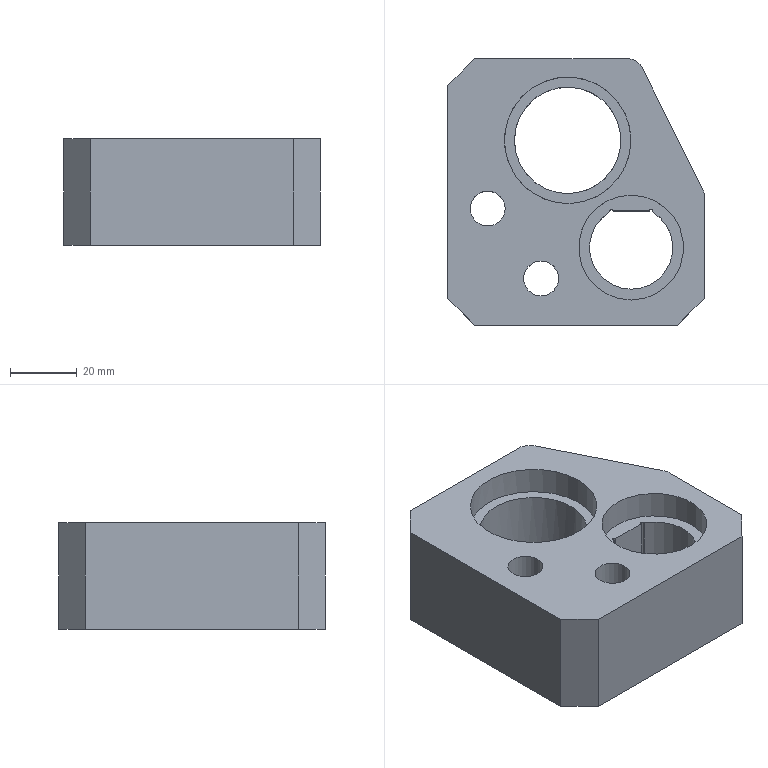Part | STEP file | lll_id3606_x_t | 1 solid | 28 faces | box 77 x 80 x 32 mm | volume 124628 mm3 | plane 15 | cylinder 13 | commonest cylinder face diameters 1 x2 10 x2 10.5 x2 17 x2 25 x2 31.5 x1
STEP:
#1=CARTESIAN_POINT('',(3364.435,-91.25,84.3));
#2=VERTEX_POINT('',#1);
#3=CARTESIAN_POINT('',(3364.435,-75.5,84.3));
#4=DIRECTION('',(0.,0.,-1.));
#5=DIRECTION('',(1.,0.,0.));
#6=AXIS2_PLACEMENT_3D('',#3,#4,#5);
#7=CIRCLE('',#6,15.75);
#8=EDGE_CURVE('',#2,#2,#7,.T.);
#9=ORIENTED_EDGE('',*,*,#8,.F.);
#10=EDGE_LOOP('',(#9));
#11=FACE_BOUND('',#10,.T.);
#12=CARTESIAN_POINT('',(3370.807,-64.746,84.3));
#13=VERTEX_POINT('',#12);
#14=CARTESIAN_POINT('',(3369.872,-64.5,84.3));
#15=VERTEX_POINT('',#14);
#16=CARTESIAN_POINT('',(3370.372,-64.5,84.3));
#17=DIRECTION('',(0.,0.,1.));
#18=DIRECTION('',(-1.,0.,0.));
#19=AXIS2_PLACEMENT_3D('',#16,#17,#18);
#20=CIRCLE('',#19,0.5);
#21=EDGE_CURVE('',#13,#15,#20,.T.);
#22=ORIENTED_EDGE('',*,*,#21,.F.);
#23=CARTESIAN_POINT('',(3364.435,-88.,84.3));
#24=VERTEX_POINT('',#23);
#25=CARTESIAN_POINT('',(3364.435,-75.5,84.3));
#26=DIRECTION('',(0.,0.,-1.));
#27=DIRECTION('',(-1.,0.,0.));
#28=AXIS2_PLACEMENT_3D('',#25,#26,#27);
#29=CIRCLE('',#28,12.5);
#30=EDGE_CURVE('',#13,#24,#29,.T.);
#31=ORIENTED_EDGE('',*,*,#30,.T.);
#32=CARTESIAN_POINT('',(3358.063,-64.746,84.3));
#33=VERTEX_POINT('',#32);
#34=CARTESIAN_POINT('',(3364.435,-75.5,84.3));
#35=DIRECTION('',(0.,0.,-1.));
#36=DIRECTION('',(-1.,0.,0.));
#37=AXIS2_PLACEMENT_3D('',#34,#35,#36);
#38=CIRCLE('',#37,12.5);
#39=EDGE_CURVE('',#24,#33,#38,.T.);
#40=ORIENTED_EDGE('',*,*,#39,.T.);
#41=CARTESIAN_POINT('',(3358.998,-64.5,84.3));
#42=VERTEX_POINT('',#41);
#43=CARTESIAN_POINT('',(3358.498,-64.5,84.3));
#44=DIRECTION('',(0.,0.,-1.));
#45=DIRECTION('',(1.,0.,0.));
#46=AXIS2_PLACEMENT_3D('',#43,#44,#45);
#47=CIRCLE('',#46,0.5);
#48=EDGE_CURVE('',#33,#42,#47,.T.);
#49=ORIENTED_EDGE('',*,*,#48,.T.);
#50=CARTESIAN_POINT('',(3345.367,-64.5,84.3));
#51=DIRECTION('',(1.,0.,0.));
#52=VECTOR('',#51,1.);
#53=LINE('',#50,#52);
#54=EDGE_CURVE('',#42,#15,#53,.T.);
#55=ORIENTED_EDGE('',*,*,#54,.T.);
#56=EDGE_LOOP('',(#22,#31,#40,#49,#55));
#57=FACE_BOUND('',#56,.T.);
#58=CARTESIAN_POINT('',(3345.367,-52.038,84.3));
#59=DIRECTION('',(0.,0.,-1.));
#60=DIRECTION('',(0.,-1.,0.));
#61=AXIS2_PLACEMENT_3D('',#58,#59,#60);
#62=PLANE('',#61);
#63=ADVANCED_FACE('',(#11,#57),#62,.F.);
#64=CARTESIAN_POINT('',(3316.117,-63.788,77.5));
#65=VERTEX_POINT('',#64);
#66=CARTESIAN_POINT('',(3321.367,-63.788,77.5));
#67=DIRECTION('',(0.,0.,-1.));
#68=DIRECTION('',(-1.,0.,0.));
#69=AXIS2_PLACEMENT_3D('',#66,#67,#68);
#70=CIRCLE('',#69,5.25);
#71=EDGE_CURVE('',#65,#65,#70,.T.);
#72=ORIENTED_EDGE('',*,*,#71,.F.);
#73=EDGE_LOOP('',(#72));
#74=FACE_BOUND('',#73,.T.);
#75=CARTESIAN_POINT('',(3312.867,-63.788,77.5));
#76=VERTEX_POINT('',#75);
#77=CARTESIAN_POINT('',(3321.367,-63.788,77.5));
#78=DIRECTION('',(0.,0.,-1.));
#79=DIRECTION('',(-1.,0.,0.));
#80=AXIS2_PLACEMENT_3D('',#77,#78,#79);
#81=CIRCLE('',#80,8.5);
#82=EDGE_CURVE('',#76,#76,#81,.T.);
#83=ORIENTED_EDGE('',*,*,#82,.T.);
#84=EDGE_LOOP('',(#83));
#85=FACE_BOUND('',#84,.T.);
#86=CARTESIAN_POINT('',(3321.367,-63.788,77.5));
#87=DIRECTION('',(0.,0.,1.));
#88=DIRECTION('',(-1.,0.,0.));
#89=AXIS2_PLACEMENT_3D('',#86,#87,#88);
#90=PLANE('',#89);
#91=ADVANCED_FACE('',(#74,#85),#90,.F.);
#92=CARTESIAN_POINT('',(3326.367,-43.288,84.3));
#93=VERTEX_POINT('',#92);
#94=CARTESIAN_POINT('',(3345.367,-43.288,84.3));
#95=DIRECTION('',(0.,0.,-1.));
#96=DIRECTION('',(-1.,0.,0.));
#97=AXIS2_PLACEMENT_3D('',#94,#95,#96);
#98=CIRCLE('',#97,19.);
#99=EDGE_CURVE('',#93,#93,#98,.T.);
#100=ORIENTED_EDGE('',*,*,#99,.F.);
#101=EDGE_LOOP('',(#100));
#102=FACE_BOUND('',#101,.T.);
#103=CARTESIAN_POINT('',(3329.367,-43.288,84.3));
#104=VERTEX_POINT('',#103);
#105=CARTESIAN_POINT('',(3345.367,-43.288,84.3));
#106=DIRECTION('',(0.,0.,-1.));
#107=DIRECTION('',(-1.,0.,0.));
#108=AXIS2_PLACEMENT_3D('',#105,#106,#107);
#109=CIRCLE('',#108,16.);
#110=EDGE_CURVE('',#104,#104,#109,.T.);
#111=ORIENTED_EDGE('',*,*,#110,.T.);
#112=EDGE_LOOP('',(#111));
#113=FACE_BOUND('',#112,.T.);
#114=CARTESIAN_POINT('',(3345.367,-52.038,84.3));
#115=DIRECTION('',(0.,0.,-1.));
#116=DIRECTION('',(0.,-1.,0.));
#117=AXIS2_PLACEMENT_3D('',#114,#115,#116);
#118=PLANE('',#117);
#119=ADVANCED_FACE('',(#102,#113),#118,.F.);
#120=ORIENTED_EDGE('',*,*,#82,.F.);
#121=EDGE_LOOP('',(#120));
#122=FACE_BOUND('',#121,.T.);
#123=CARTESIAN_POINT('',(3312.867,-63.788,60.5));
#124=VERTEX_POINT('',#123);
#125=CARTESIAN_POINT('',(3321.367,-63.788,60.5));
#126=DIRECTION('',(0.,0.,1.));
#127=DIRECTION('',(-1.,0.,0.));
#128=AXIS2_PLACEMENT_3D('',#125,#126,#127);
#129=CIRCLE('',#128,8.5);
#130=EDGE_CURVE('',#124,#124,#129,.T.);
#131=ORIENTED_EDGE('',*,*,#130,.F.);
#132=EDGE_LOOP('',(#131));
#133=FACE_BOUND('',#132,.T.);
#134=CARTESIAN_POINT('',(3321.367,-63.788,60.5));
#135=DIRECTION('',(0.,0.,1.));
#136=DIRECTION('',(-1.,0.,0.));
#137=AXIS2_PLACEMENT_3D('',#134,#135,#136);
#138=CYLINDRICAL_SURFACE('',#137,8.5);
#139=ADVANCED_FACE('',(#122,#133),#138,.F.);
#140=CARTESIAN_POINT('',(3385.838,-57.732,92.5));
#141=VERTEX_POINT('',#140);
#142=CARTESIAN_POINT('',(3386.366,-59.968,92.5));
#143=VERTEX_POINT('',#142);
#144=CARTESIAN_POINT('',(3381.366,-59.968,92.5));
#145=DIRECTION('',(0.,0.,-1.));
#146=DIRECTION('',(-1.,0.,0.));
#147=AXIS2_PLACEMENT_3D('',#144,#145,#146);
#148=CIRCLE('',#147,5.);
#149=EDGE_CURVE('',#141,#143,#148,.T.);
#150=ORIENTED_EDGE('',*,*,#149,.T.);
#151=CARTESIAN_POINT('',(3386.366,-59.968,60.5));
#152=VERTEX_POINT('',#151);
#153=CARTESIAN_POINT('',(3386.366,-59.968,-8.5));
#154=DIRECTION('',(0.,0.,-1.));
#155=VECTOR('',#154,1.);
#156=LINE('',#153,#155);
#157=EDGE_CURVE('',#143,#152,#156,.T.);
#158=ORIENTED_EDGE('',*,*,#157,.T.);
#159=CARTESIAN_POINT('',(3385.838,-57.732,60.5));
#160=VERTEX_POINT('',#159);
#161=CARTESIAN_POINT('',(3381.366,-59.968,60.5));
#162=DIRECTION('',(0.,0.,1.));
#163=DIRECTION('',(-1.,0.,0.));
#164=AXIS2_PLACEMENT_3D('',#161,#162,#163);
#165=CIRCLE('',#164,5.);
#166=EDGE_CURVE('',#152,#160,#165,.T.);
#167=ORIENTED_EDGE('',*,*,#166,.T.);
#168=CARTESIAN_POINT('',(3385.838,-57.732,-8.5));
#169=DIRECTION('',(0.,0.,1.));
#170=VECTOR('',#169,1.);
#171=LINE('',#168,#170);
#172=EDGE_CURVE('',#160,#141,#171,.T.);
#173=ORIENTED_EDGE('',*,*,#172,.T.);
#174=EDGE_LOOP('',(#150,#158,#167,#173));
#175=FACE_OUTER_BOUND('',#174,.T.);
#176=CARTESIAN_POINT('',(3381.366,-59.968,-8.5));
#177=DIRECTION('',(0.,0.,1.));
#178=DIRECTION('',(-1.,0.,0.));
#179=AXIS2_PLACEMENT_3D('',#176,#177,#178);
#180=CYLINDRICAL_SURFACE('',#179,5.);
#181=ADVANCED_FACE('',(#175),#180,.T.);
#182=CARTESIAN_POINT('',(3386.366,-90.788,92.5));
#183=VERTEX_POINT('',#182);
#184=CARTESIAN_POINT('',(3386.366,-69.563,92.5));
#185=DIRECTION('',(0.,-1.,0.));
#186=VECTOR('',#185,1.);
#187=LINE('',#184,#186);
#188=EDGE_CURVE('',#143,#183,#187,.T.);
#189=ORIENTED_EDGE('',*,*,#188,.T.);
#190=CARTESIAN_POINT('',(3386.366,-90.788,60.5));
#191=VERTEX_POINT('',#190);
#192=CARTESIAN_POINT('',(3386.366,-90.788,-8.5));
#193=DIRECTION('',(0.,0.,1.));
#194=VECTOR('',#193,1.);
#195=LINE('',#192,#194);
#196=EDGE_CURVE('',#191,#183,#195,.T.);
#197=ORIENTED_EDGE('',*,*,#196,.F.);
#198=CARTESIAN_POINT('',(3386.366,-69.563,60.5));
#199=DIRECTION('',(0.,1.,0.));
#200=VECTOR('',#199,1.);
#201=LINE('',#198,#200);
#202=EDGE_CURVE('',#191,#152,#201,.T.);
#203=ORIENTED_EDGE('',*,*,#202,.T.);
#204=ORIENTED_EDGE('',*,*,#157,.F.);
#205=EDGE_LOOP('',(#189,#197,#203,#204));
#206=FACE_OUTER_BOUND('',#205,.T.);
#207=CARTESIAN_POINT('',(3386.366,-38.338,-8.5));
#208=DIRECTION('',(1.,0.,0.));
#209=DIRECTION('',(0.,0.,1.));
#210=AXIS2_PLACEMENT_3D('',#207,#208,#209);
#211=PLANE('',#210);
#212=ADVANCED_FACE('',(#206),#211,.T.);
#213=CARTESIAN_POINT('',(3378.366,-98.788,60.5));
#214=VERTEX_POINT('',#213);
#215=CARTESIAN_POINT('',(3344.383,-132.771,60.5));
#216=DIRECTION('',(0.7071,0.7071,0.));
#217=VECTOR('',#216,1.);
#218=LINE('',#215,#217);
#219=EDGE_CURVE('',#214,#191,#218,.T.);
#220=ORIENTED_EDGE('',*,*,#219,.T.);
#221=ORIENTED_EDGE('',*,*,#196,.T.);
#222=CARTESIAN_POINT('',(3378.366,-98.788,92.5));
#223=VERTEX_POINT('',#222);
#224=CARTESIAN_POINT('',(3339.434,-137.72,92.5));
#225=DIRECTION('',(-0.7071,-0.7071,0.));
#226=VECTOR('',#225,1.);
#227=LINE('',#224,#226);
#228=EDGE_CURVE('',#183,#223,#227,.T.);
#229=ORIENTED_EDGE('',*,*,#228,.T.);
#230=CARTESIAN_POINT('',(3378.366,-98.788,-8.5));
#231=DIRECTION('',(0.,0.,-1.));
#232=VECTOR('',#231,1.);
#233=LINE('',#230,#232);
#234=EDGE_CURVE('',#223,#214,#233,.T.);
#235=ORIENTED_EDGE('',*,*,#234,.T.);
#236=EDGE_LOOP('',(#220,#221,#229,#235));
#237=FACE_OUTER_BOUND('',#236,.T.);
#238=CARTESIAN_POINT('',(3386.366,-90.788,-8.5));
#239=DIRECTION('',(-0.7071,0.7071,0.));
#240=DIRECTION('',(0.,0.,1.));
#241=AXIS2_PLACEMENT_3D('',#238,#239,#240);
#242=PLANE('',#241);
#243=ADVANCED_FACE('',(#237),#242,.F.);
#244=CARTESIAN_POINT('',(3317.367,-98.788,92.5));
#245=VERTEX_POINT('',#244);
#246=CARTESIAN_POINT('',(3345.367,-98.788,92.5));
#247=DIRECTION('',(-1.,0.,0.));
#248=VECTOR('',#247,1.);
#249=LINE('',#246,#248);
#250=EDGE_CURVE('',#223,#245,#249,.T.);
#251=ORIENTED_EDGE('',*,*,#250,.T.);
#252=CARTESIAN_POINT('',(3317.367,-98.788,60.5));
#253=VERTEX_POINT('',#252);
#254=CARTESIAN_POINT('',(3317.367,-98.788,-8.5));
#255=DIRECTION('',(0.,0.,1.));
#256=VECTOR('',#255,1.);
#257=LINE('',#254,#256);
#258=EDGE_CURVE('',#253,#245,#257,.T.);
#259=ORIENTED_EDGE('',*,*,#258,.F.);
#260=CARTESIAN_POINT('',(3282.176,-98.788,60.5));
#261=DIRECTION('',(1.,0.,0.));
#262=VECTOR('',#261,1.);
#263=LINE('',#260,#262);
#264=EDGE_CURVE('',#253,#214,#263,.T.);
#265=ORIENTED_EDGE('',*,*,#264,.T.);
#266=ORIENTED_EDGE('',*,*,#234,.F.);
#267=EDGE_LOOP('',(#251,#259,#265,#266));
#268=FACE_OUTER_BOUND('',#267,.T.);
#269=CARTESIAN_POINT('',(3345.367,-98.788,-8.5));
#270=DIRECTION('',(0.,-1.,0.));
#271=DIRECTION('',(0.,0.,1.));
#272=AXIS2_PLACEMENT_3D('',#269,#270,#271);
#273=PLANE('',#272);
#274=ADVANCED_FACE('',(#268),#273,.T.);
#275=CARTESIAN_POINT('',(3309.367,-90.788,60.5));
#276=VERTEX_POINT('',#275);
#277=CARTESIAN_POINT('',(3280.659,-62.08,60.5));
#278=DIRECTION('',(0.7071,-0.7071,0.));
#279=VECTOR('',#278,1.);
#280=LINE('',#277,#279);
#281=EDGE_CURVE('',#276,#253,#280,.T.);
#282=ORIENTED_EDGE('',*,*,#281,.T.);
#283=ORIENTED_EDGE('',*,*,#258,.T.);
#284=CARTESIAN_POINT('',(3309.367,-90.788,92.5));
#285=VERTEX_POINT('',#284);
#286=CARTESIAN_POINT('',(3280.659,-62.08,92.5));
#287=DIRECTION('',(-0.7071,0.7071,0.));
#288=VECTOR('',#287,1.);
#289=LINE('',#286,#288);
#290=EDGE_CURVE('',#245,#285,#289,.T.);
#291=ORIENTED_EDGE('',*,*,#290,.T.);
#292=CARTESIAN_POINT('',(3309.367,-90.788,-8.5));
#293=DIRECTION('',(0.,0.,-1.));
#294=VECTOR('',#293,1.);
#295=LINE('',#292,#294);
#296=EDGE_CURVE('',#285,#276,#295,.T.);
#297=ORIENTED_EDGE('',*,*,#296,.T.);
#298=EDGE_LOOP('',(#282,#283,#291,#297));
#299=FACE_OUTER_BOUND('',#298,.T.);
#300=CARTESIAN_POINT('',(3317.367,-98.788,-8.5));
#301=DIRECTION('',(0.7071,0.7071,0.));
#302=DIRECTION('',(0.,0.,1.));
#303=AXIS2_PLACEMENT_3D('',#300,#301,#302);
#304=PLANE('',#303);
#305=ADVANCED_FACE('',(#299),#304,.F.);
#306=CARTESIAN_POINT('',(3309.367,-26.788,92.5));
#307=VERTEX_POINT('',#306);
#308=CARTESIAN_POINT('',(3309.367,-74.513,92.5));
#309=DIRECTION('',(0.,1.,0.));
#310=VECTOR('',#309,1.);
#311=LINE('',#308,#310);
#312=EDGE_CURVE('',#285,#307,#311,.T.);
#313=ORIENTED_EDGE('',*,*,#312,.T.);
#314=CARTESIAN_POINT('',(3309.367,-26.788,60.5));
#315=VERTEX_POINT('',#314);
#316=CARTESIAN_POINT('',(3309.367,-26.788,-8.5));
#317=DIRECTION('',(0.,0.,1.));
#318=VECTOR('',#317,1.);
#319=LINE('',#316,#318);
#320=EDGE_CURVE('',#315,#307,#319,.T.);
#321=ORIENTED_EDGE('',*,*,#320,.F.);
#322=CARTESIAN_POINT('',(3309.367,-69.563,60.5));
#323=DIRECTION('',(0.,-1.,0.));
#324=VECTOR('',#323,1.);
#325=LINE('',#322,#324);
#326=EDGE_CURVE('',#315,#276,#325,.T.);
#327=ORIENTED_EDGE('',*,*,#326,.T.);
#328=ORIENTED_EDGE('',*,*,#296,.F.);
#329=EDGE_LOOP('',(#313,#321,#327,#328));
#330=FACE_OUTER_BOUND('',#329,.T.);
#331=CARTESIAN_POINT('',(3309.367,-43.288,-8.5));
#332=DIRECTION('',(-1.,0.,0.));
#333=DIRECTION('',(0.,0.,-1.));
#334=AXIS2_PLACEMENT_3D('',#331,#332,#333);
#335=PLANE('',#334);
#336=ADVANCED_FACE('',(#330),#335,.T.);
#337=CARTESIAN_POINT('',(3317.367,-18.788,60.5));
#338=VERTEX_POINT('',#337);
#339=CARTESIAN_POINT('',(3268.884,-67.271,60.5));
#340=DIRECTION('',(-0.7071,-0.7071,0.));
#341=VECTOR('',#340,1.);
#342=LINE('',#339,#341);
#343=EDGE_CURVE('',#338,#315,#342,.T.);
#344=ORIENTED_EDGE('',*,*,#343,.T.);
#345=ORIENTED_EDGE('',*,*,#320,.T.);
#346=CARTESIAN_POINT('',(3317.367,-18.788,92.5));
#347=VERTEX_POINT('',#346);
#348=CARTESIAN_POINT('',(3263.934,-72.22,92.5));
#349=DIRECTION('',(0.7071,0.7071,0.));
#350=VECTOR('',#349,1.);
#351=LINE('',#348,#350);
#352=EDGE_CURVE('',#307,#347,#351,.T.);
#353=ORIENTED_EDGE('',*,*,#352,.T.);
#354=CARTESIAN_POINT('',(3317.367,-18.788,-8.5));
#355=DIRECTION('',(0.,0.,-1.));
#356=VECTOR('',#355,1.);
#357=LINE('',#354,#356);
#358=EDGE_CURVE('',#347,#338,#357,.T.);
#359=ORIENTED_EDGE('',*,*,#358,.T.);
#360=EDGE_LOOP('',(#344,#345,#353,#359));
#361=FACE_OUTER_BOUND('',#360,.T.);
#362=CARTESIAN_POINT('',(3309.367,-26.788,-8.5));
#363=DIRECTION('',(0.7071,-0.7071,0.));
#364=DIRECTION('',(0.,0.,1.));
#365=AXIS2_PLACEMENT_3D('',#362,#363,#364);
#366=PLANE('',#365);
#367=ADVANCED_FACE('',(#361),#366,.F.);
#368=CARTESIAN_POINT('',(3363.276,-18.788,60.5));
#369=VERTEX_POINT('',#368);
#370=CARTESIAN_POINT('',(3282.176,-18.788,60.5));
#371=DIRECTION('',(-1.,0.,0.));
#372=VECTOR('',#371,1.);
#373=LINE('',#370,#372);
#374=EDGE_CURVE('',#369,#338,#373,.T.);
#375=ORIENTED_EDGE('',*,*,#374,.T.);
#376=ORIENTED_EDGE('',*,*,#358,.F.);
#377=CARTESIAN_POINT('',(3363.276,-18.788,92.5));
#378=VERTEX_POINT('',#377);
#379=CARTESIAN_POINT('',(3345.367,-18.788,92.5));
#380=DIRECTION('',(1.,0.,0.));
#381=VECTOR('',#380,1.);
#382=LINE('',#379,#381);
#383=EDGE_CURVE('',#347,#378,#382,.T.);
#384=ORIENTED_EDGE('',*,*,#383,.T.);
#385=CARTESIAN_POINT('',(3363.276,-18.788,-8.5));
#386=DIRECTION('',(0.,0.,1.));
#387=VECTOR('',#386,1.);
#388=LINE('',#385,#387);
#389=EDGE_CURVE('',#369,#378,#388,.T.);
#390=ORIENTED_EDGE('',*,*,#389,.F.);
#391=EDGE_LOOP('',(#375,#376,#384,#390));
#392=FACE_OUTER_BOUND('',#391,.T.);
#393=CARTESIAN_POINT('',(3345.367,-18.788,-8.5));
#394=DIRECTION('',(0.,1.,0.));
#395=DIRECTION('',(0.,0.,-1.));
#396=AXIS2_PLACEMENT_3D('',#393,#394,#395);
#397=PLANE('',#396);
#398=ADVANCED_FACE('',(#392),#397,.T.);
#399=CARTESIAN_POINT('',(3367.748,-21.552,60.5));
#400=VERTEX_POINT('',#399);
#401=CARTESIAN_POINT('',(3363.276,-23.788,60.5));
#402=DIRECTION('',(0.,0.,1.));
#403=DIRECTION('',(-1.,0.,0.));
#404=AXIS2_PLACEMENT_3D('',#401,#402,#403);
#405=CIRCLE('',#404,5.);
#406=EDGE_CURVE('',#400,#369,#405,.T.);
#407=ORIENTED_EDGE('',*,*,#406,.T.);
#408=ORIENTED_EDGE('',*,*,#389,.T.);
#409=CARTESIAN_POINT('',(3367.748,-21.552,92.5));
#410=VERTEX_POINT('',#409);
#411=CARTESIAN_POINT('',(3363.276,-23.788,92.5));
#412=DIRECTION('',(0.,0.,-1.));
#413=DIRECTION('',(-1.,0.,0.));
#414=AXIS2_PLACEMENT_3D('',#411,#412,#413);
#415=CIRCLE('',#414,5.);
#416=EDGE_CURVE('',#378,#410,#415,.T.);
#417=ORIENTED_EDGE('',*,*,#416,.T.);
#418=CARTESIAN_POINT('',(3367.748,-21.552,-8.5));
#419=DIRECTION('',(0.,0.,-1.));
#420=VECTOR('',#419,1.);
#421=LINE('',#418,#420);
#422=EDGE_CURVE('',#410,#400,#421,.T.);
#423=ORIENTED_EDGE('',*,*,#422,.T.);
#424=EDGE_LOOP('',(#407,#408,#417,#423));
#425=FACE_OUTER_BOUND('',#424,.T.);
#426=CARTESIAN_POINT('',(3363.276,-23.788,-8.5));
#427=DIRECTION('',(0.,0.,-1.));
#428=DIRECTION('',(1.,0.,0.));
#429=AXIS2_PLACEMENT_3D('',#426,#427,#428);
#430=CYLINDRICAL_SURFACE('',#429,5.);
#431=ADVANCED_FACE('',(#425),#430,.T.);
#432=CARTESIAN_POINT('',(3370.039,-26.132,60.5));
#433=DIRECTION('',(-0.4472,0.8944,0.));
#434=VECTOR('',#433,1.);
#435=LINE('',#432,#434);
#436=EDGE_CURVE('',#160,#400,#435,.T.);
#437=ORIENTED_EDGE('',*,*,#436,.T.);
#438=ORIENTED_EDGE('',*,*,#422,.F.);
#439=CARTESIAN_POINT('',(3371.029,-28.112,92.5));
#440=DIRECTION('',(0.4472,-0.8944,0.));
#441=VECTOR('',#440,1.);
#442=LINE('',#439,#441);
#443=EDGE_CURVE('',#410,#141,#442,.T.);
#444=ORIENTED_EDGE('',*,*,#443,.T.);
#445=ORIENTED_EDGE('',*,*,#172,.F.);
#446=EDGE_LOOP('',(#437,#438,#444,#445));
#447=FACE_OUTER_BOUND('',#446,.T.);
#448=CARTESIAN_POINT('',(3386.366,-58.788,-8.5));
#449=DIRECTION('',(-0.8944,-0.4472,0.));
#450=DIRECTION('',(0.,0.,-1.));
#451=AXIS2_PLACEMENT_3D('',#448,#449,#450);
#452=PLANE('',#451);
#453=ADVANCED_FACE('',(#447),#452,.F.);
#454=CARTESIAN_POINT('',(3316.117,-63.788,92.5));
#455=VERTEX_POINT('',#454);
#456=CARTESIAN_POINT('',(3321.367,-63.788,92.5));
#457=DIRECTION('',(0.,0.,1.));
#458=DIRECTION('',(-1.,0.,0.));
#459=AXIS2_PLACEMENT_3D('',#456,#457,#458);
#460=CIRCLE('',#459,5.25);
#461=EDGE_CURVE('',#455,#455,#460,.T.);
#462=ORIENTED_EDGE('',*,*,#461,.T.);
#463=EDGE_LOOP('',(#462));
#464=FACE_BOUND('',#463,.T.);
#465=ORIENTED_EDGE('',*,*,#71,.T.);
#466=EDGE_LOOP('',(#465));
#467=FACE_BOUND('',#466,.T.);
#468=CARTESIAN_POINT('',(3321.367,-63.788,160.5));
#469=DIRECTION('',(0.,0.,1.));
#470=DIRECTION('',(-1.,0.,0.));
#471=AXIS2_PLACEMENT_3D('',#468,#469,#470);
#472=CYLINDRICAL_SURFACE('',#471,5.25);
#473=ADVANCED_FACE('',(#464,#467),#472,.F.);
#474=CARTESIAN_POINT('',(3364.367,-43.288,92.5));
#475=VERTEX_POINT('',#474);
#476=CARTESIAN_POINT('',(3345.367,-43.288,92.5));
#477=DIRECTION('',(0.,0.,1.));
#478=DIRECTION('',(1.,0.,0.));
#479=AXIS2_PLACEMENT_3D('',#476,#477,#478);
#480=CIRCLE('',#479,19.);
#481=EDGE_CURVE('',#475,#475,#480,.T.);
#482=ORIENTED_EDGE('',*,*,#481,.T.);
#483=EDGE_LOOP('',(#482));
#484=FACE_BOUND('',#483,.T.);
#485=ORIENTED_EDGE('',*,*,#99,.T.);
#486=EDGE_LOOP('',(#485));
#487=FACE_BOUND('',#486,.T.);
#488=CARTESIAN_POINT('',(3345.367,-43.288,90.));
#489=DIRECTION('',(0.,0.,-1.));
#490=DIRECTION('',(0.,1.,0.));
#491=AXIS2_PLACEMENT_3D('',#488,#489,#490);
#492=CYLINDRICAL_SURFACE('',#491,19.);
#493=ADVANCED_FACE('',(#484,#487),#492,.F.);
#494=CARTESIAN_POINT('',(3364.435,-91.25,92.5));
#495=VERTEX_POINT('',#494);
#496=CARTESIAN_POINT('',(3364.435,-75.5,92.5));
#497=DIRECTION('',(0.,0.,1.));
#498=DIRECTION('',(-1.,0.,0.));
#499=AXIS2_PLACEMENT_3D('',#496,#497,#498);
#500=CIRCLE('',#499,15.75);
#501=EDGE_CURVE('',#495,#495,#500,.T.);
#502=ORIENTED_EDGE('',*,*,#501,.T.);
#503=CARTESIAN_POINT('',(3364.435,-91.25,88.5));
#504=DIRECTION('',(0.,0.,-1.));
#505=VECTOR('',#504,1.);
#506=LINE('',#503,#505);
#507=EDGE_CURVE('',#495,#2,#506,.T.);
#508=ORIENTED_EDGE('',*,*,#507,.T.);
#509=ORIENTED_EDGE('',*,*,#8,.T.);
#510=ORIENTED_EDGE('',*,*,#507,.F.);
#511=EDGE_LOOP('',(#502,#508,#509,#510));
#512=FACE_OUTER_BOUND('',#511,.T.);
#513=CARTESIAN_POINT('',(3364.435,-75.5,88.5));
#514=DIRECTION('',(0.,0.,-1.));
#515=DIRECTION('',(0.,1.,0.));
#516=AXIS2_PLACEMENT_3D('',#513,#514,#515);
#517=CYLINDRICAL_SURFACE('',#516,15.75);
#518=ADVANCED_FACE('',(#512),#517,.F.);
#519=CARTESIAN_POINT('',(3342.617,-84.788,92.5));
#520=VERTEX_POINT('',#519);
#521=CARTESIAN_POINT('',(3337.367,-84.788,92.5));
#522=DIRECTION('',(0.,0.,1.));
#523=DIRECTION('',(1.,0.,0.));
#524=AXIS2_PLACEMENT_3D('',#521,#522,#523);
#525=CIRCLE('',#524,5.25);
#526=EDGE_CURVE('',#520,#520,#525,.T.);
#527=ORIENTED_EDGE('',*,*,#526,.F.);
#528=EDGE_LOOP('',(#527));
#529=FACE_BOUND('',#528,.T.);
#530=ORIENTED_EDGE('',*,*,#501,.F.);
#531=EDGE_LOOP('',(#530));
#532=FACE_BOUND('',#531,.T.);
#533=ORIENTED_EDGE('',*,*,#481,.F.);
#534=EDGE_LOOP('',(#533));
#535=FACE_BOUND('',#534,.T.);
#536=ORIENTED_EDGE('',*,*,#461,.F.);
#537=EDGE_LOOP('',(#536));
#538=FACE_BOUND('',#537,.T.);
#539=ORIENTED_EDGE('',*,*,#443,.F.);
#540=ORIENTED_EDGE('',*,*,#416,.F.);
#541=ORIENTED_EDGE('',*,*,#383,.F.);
#542=ORIENTED_EDGE('',*,*,#352,.F.);
#543=ORIENTED_EDGE('',*,*,#312,.F.);
#544=ORIENTED_EDGE('',*,*,#290,.F.);
#545=ORIENTED_EDGE('',*,*,#250,.F.);
#546=ORIENTED_EDGE('',*,*,#228,.F.);
#547=ORIENTED_EDGE('',*,*,#188,.F.);
#548=ORIENTED_EDGE('',*,*,#149,.F.);
#549=EDGE_LOOP('',(#539,#540,#541,#542,#543,#544,#545,#546,#547,#548));
#550=FACE_BOUND('',#549,.T.);
#551=CARTESIAN_POINT('',(3277.227,-74.513,92.5));
#552=DIRECTION('',(0.,0.,1.));
#553=DIRECTION('',(-1.,0.,0.));
#554=AXIS2_PLACEMENT_3D('',#551,#552,#553);
#555=PLANE('',#554);
#556=ADVANCED_FACE('',(#529,#532,#535,#538,#550),#555,.T.);
#557=CARTESIAN_POINT('',(3361.367,-43.288,60.5));
#558=VERTEX_POINT('',#557);
#559=CARTESIAN_POINT('',(3345.367,-43.288,60.5));
#560=DIRECTION('',(0.,0.,-1.));
#561=DIRECTION('',(1.,0.,0.));
#562=AXIS2_PLACEMENT_3D('',#559,#560,#561);
#563=CIRCLE('',#562,16.);
#564=EDGE_CURVE('',#558,#558,#563,.T.);
#565=ORIENTED_EDGE('',*,*,#564,.T.);
#566=EDGE_LOOP('',(#565));
#567=FACE_BOUND('',#566,.T.);
#568=ORIENTED_EDGE('',*,*,#110,.F.);
#569=EDGE_LOOP('',(#568));
#570=FACE_BOUND('',#569,.T.);
#571=CARTESIAN_POINT('',(3345.367,-43.288,44.8));
#572=DIRECTION('',(0.,0.,-1.));
#573=DIRECTION('',(0.,1.,0.));
#574=AXIS2_PLACEMENT_3D('',#571,#572,#573);
#575=CYLINDRICAL_SURFACE('',#574,16.);
#576=ADVANCED_FACE('',(#567,#570),#575,.F.);
#577=CARTESIAN_POINT('',(3369.872,-64.5,60.5));
#578=VERTEX_POINT('',#577);
#579=CARTESIAN_POINT('',(3370.807,-64.746,60.5));
#580=VERTEX_POINT('',#579);
#581=CARTESIAN_POINT('',(3370.372,-64.5,60.5));
#582=DIRECTION('',(0.,0.,-1.));
#583=DIRECTION('',(1.,0.,0.));
#584=AXIS2_PLACEMENT_3D('',#581,#582,#583);
#585=CIRCLE('',#584,0.5);
#586=EDGE_CURVE('',#578,#580,#585,.T.);
#587=ORIENTED_EDGE('',*,*,#586,.F.);
#588=CARTESIAN_POINT('',(3358.998,-64.5,60.5));
#589=VERTEX_POINT('',#588);
#590=CARTESIAN_POINT('',(3282.176,-64.5,60.5));
#591=DIRECTION('',(1.,0.,0.));
#592=VECTOR('',#591,1.);
#593=LINE('',#590,#592);
#594=EDGE_CURVE('',#589,#578,#593,.T.);
#595=ORIENTED_EDGE('',*,*,#594,.F.);
#596=CARTESIAN_POINT('',(3358.063,-64.746,60.5));
#597=VERTEX_POINT('',#596);
#598=CARTESIAN_POINT('',(3358.498,-64.5,60.5));
#599=DIRECTION('',(0.,0.,-1.));
#600=DIRECTION('',(1.,0.,0.));
#601=AXIS2_PLACEMENT_3D('',#598,#599,#600);
#602=CIRCLE('',#601,0.5);
#603=EDGE_CURVE('',#597,#589,#602,.T.);
#604=ORIENTED_EDGE('',*,*,#603,.F.);
#605=CARTESIAN_POINT('',(3364.435,-88.,60.5));
#606=VERTEX_POINT('',#605);
#607=CARTESIAN_POINT('',(3364.435,-75.5,60.5));
#608=DIRECTION('',(0.,0.,-1.));
#609=DIRECTION('',(1.,0.,0.));
#610=AXIS2_PLACEMENT_3D('',#607,#608,#609);
#611=CIRCLE('',#610,12.5);
#612=EDGE_CURVE('',#606,#597,#611,.T.);
#613=ORIENTED_EDGE('',*,*,#612,.F.);
#614=CARTESIAN_POINT('',(3364.435,-75.5,60.5));
#615=DIRECTION('',(0.,0.,-1.));
#616=DIRECTION('',(1.,0.,0.));
#617=AXIS2_PLACEMENT_3D('',#614,#615,#616);
#618=CIRCLE('',#617,12.5);
#619=EDGE_CURVE('',#580,#606,#618,.T.);
#620=ORIENTED_EDGE('',*,*,#619,.F.);
#621=EDGE_LOOP('',(#587,#595,#604,#613,#620));
#622=FACE_BOUND('',#621,.T.);
#623=CARTESIAN_POINT('',(3345.867,-84.788,60.5));
#624=VERTEX_POINT('',#623);
#625=CARTESIAN_POINT('',(3337.367,-84.788,60.5));
#626=DIRECTION('',(0.,0.,-1.));
#627=DIRECTION('',(1.,0.,0.));
#628=AXIS2_PLACEMENT_3D('',#625,#626,#627);
#629=CIRCLE('',#628,8.5);
#630=EDGE_CURVE('',#624,#624,#629,.T.);
#631=ORIENTED_EDGE('',*,*,#630,.F.);
#632=EDGE_LOOP('',(#631));
#633=FACE_BOUND('',#632,.T.);
#634=ORIENTED_EDGE('',*,*,#564,.F.);
#635=EDGE_LOOP('',(#634));
#636=FACE_BOUND('',#635,.T.);
#637=ORIENTED_EDGE('',*,*,#202,.F.);
#638=ORIENTED_EDGE('',*,*,#219,.F.);
#639=ORIENTED_EDGE('',*,*,#264,.F.);
#640=ORIENTED_EDGE('',*,*,#281,.F.);
#641=ORIENTED_EDGE('',*,*,#326,.F.);
#642=ORIENTED_EDGE('',*,*,#343,.F.);
#643=ORIENTED_EDGE('',*,*,#374,.F.);
#644=ORIENTED_EDGE('',*,*,#406,.F.);
#645=ORIENTED_EDGE('',*,*,#436,.F.);
#646=ORIENTED_EDGE('',*,*,#166,.F.);
#647=EDGE_LOOP('',(#637,#638,#639,#640,#641,#642,#643,#644,#645,#646));
#648=FACE_BOUND('',#647,.T.);
#649=ORIENTED_EDGE('',*,*,#130,.T.);
#650=EDGE_LOOP('',(#649));
#651=FACE_BOUND('',#650,.T.);
#652=CARTESIAN_POINT('',(3282.176,-69.563,60.5));
#653=DIRECTION('',(0.,0.,1.));
#654=DIRECTION('',(-1.,0.,0.));
#655=AXIS2_PLACEMENT_3D('',#652,#653,#654);
#656=PLANE('',#655);
#657=ADVANCED_FACE('',(#622,#633,#636,#648,#651),#656,.F.);
#658=CARTESIAN_POINT('',(3332.117,-84.788,77.5));
#659=VERTEX_POINT('',#658);
#660=CARTESIAN_POINT('',(3337.367,-84.788,77.5));
#661=DIRECTION('',(0.,0.,-1.));
#662=DIRECTION('',(-1.,0.,0.));
#663=AXIS2_PLACEMENT_3D('',#660,#661,#662);
#664=CIRCLE('',#663,5.25);
#665=EDGE_CURVE('',#659,#659,#664,.T.);
#666=ORIENTED_EDGE('',*,*,#665,.F.);
#667=EDGE_LOOP('',(#666));
#668=FACE_BOUND('',#667,.T.);
#669=CARTESIAN_POINT('',(3328.867,-84.788,77.5));
#670=VERTEX_POINT('',#669);
#671=CARTESIAN_POINT('',(3337.367,-84.788,77.5));
#672=DIRECTION('',(0.,0.,-1.));
#673=DIRECTION('',(-1.,0.,0.));
#674=AXIS2_PLACEMENT_3D('',#671,#672,#673);
#675=CIRCLE('',#674,8.5);
#676=EDGE_CURVE('',#670,#670,#675,.T.);
#677=ORIENTED_EDGE('',*,*,#676,.T.);
#678=EDGE_LOOP('',(#677));
#679=FACE_BOUND('',#678,.T.);
#680=CARTESIAN_POINT('',(3337.367,-84.788,77.5));
#681=DIRECTION('',(0.,0.,1.));
#682=DIRECTION('',(-1.,0.,0.));
#683=AXIS2_PLACEMENT_3D('',#680,#681,#682);
#684=PLANE('',#683);
#685=ADVANCED_FACE('',(#668,#679),#684,.F.);
#686=ORIENTED_EDGE('',*,*,#526,.T.);
#687=EDGE_LOOP('',(#686));
#688=FACE_BOUND('',#687,.T.);
#689=ORIENTED_EDGE('',*,*,#665,.T.);
#690=EDGE_LOOP('',(#689));
#691=FACE_BOUND('',#690,.T.);
#692=CARTESIAN_POINT('',(3337.367,-84.788,160.5));
#693=DIRECTION('',(0.,0.,1.));
#694=DIRECTION('',(-1.,0.,0.));
#695=AXIS2_PLACEMENT_3D('',#692,#693,#694);
#696=CYLINDRICAL_SURFACE('',#695,5.25);
#697=ADVANCED_FACE('',(#688,#691),#696,.F.);
#698=ORIENTED_EDGE('',*,*,#676,.F.);
#699=EDGE_LOOP('',(#698));
#700=FACE_BOUND('',#699,.T.);
#701=ORIENTED_EDGE('',*,*,#630,.T.);
#702=EDGE_LOOP('',(#701));
#703=FACE_BOUND('',#702,.T.);
#704=CARTESIAN_POINT('',(3337.367,-84.788,60.5));
#705=DIRECTION('',(0.,0.,1.));
#706=DIRECTION('',(-1.,0.,0.));
#707=AXIS2_PLACEMENT_3D('',#704,#705,#706);
#708=CYLINDRICAL_SURFACE('',#707,8.5);
#709=ADVANCED_FACE('',(#700,#703),#708,.F.);
#710=ORIENTED_EDGE('',*,*,#30,.F.);
#711=CARTESIAN_POINT('',(3370.807,-64.746,66.8));
#712=DIRECTION('',(0.,0.,-1.));
#713=VECTOR('',#712,1.);
#714=LINE('',#711,#713);
#715=EDGE_CURVE('',#13,#580,#714,.T.);
#716=ORIENTED_EDGE('',*,*,#715,.T.);
#717=ORIENTED_EDGE('',*,*,#619,.T.);
#718=CARTESIAN_POINT('',(3364.435,-88.,38.5));
#719=DIRECTION('',(0.,0.,-1.));
#720=VECTOR('',#719,1.);
#721=LINE('',#718,#720);
#722=EDGE_CURVE('',#24,#606,#721,.T.);
#723=ORIENTED_EDGE('',*,*,#722,.F.);
#724=EDGE_LOOP('',(#710,#716,#717,#723));
#725=FACE_OUTER_BOUND('',#724,.T.);
#726=CARTESIAN_POINT('',(3364.435,-75.5,38.5));
#727=DIRECTION('',(0.,0.,-1.));
#728=DIRECTION('',(0.,1.,0.));
#729=AXIS2_PLACEMENT_3D('',#726,#727,#728);
#730=CYLINDRICAL_SURFACE('',#729,12.5);
#731=ADVANCED_FACE('',(#725),#730,.F.);
#732=ORIENTED_EDGE('',*,*,#612,.T.);
#733=CARTESIAN_POINT('',(3358.063,-64.746,66.8));
#734=DIRECTION('',(0.,0.,1.));
#735=VECTOR('',#734,1.);
#736=LINE('',#733,#735);
#737=EDGE_CURVE('',#597,#33,#736,.T.);
#738=ORIENTED_EDGE('',*,*,#737,.T.);
#739=ORIENTED_EDGE('',*,*,#39,.F.);
#740=ORIENTED_EDGE('',*,*,#722,.T.);
#741=EDGE_LOOP('',(#732,#738,#739,#740));
#742=FACE_OUTER_BOUND('',#741,.T.);
#743=CARTESIAN_POINT('',(3364.435,-75.5,38.5));
#744=DIRECTION('',(0.,0.,-1.));
#745=DIRECTION('',(0.,1.,0.));
#746=AXIS2_PLACEMENT_3D('',#743,#744,#745);
#747=CYLINDRICAL_SURFACE('',#746,12.5);
#748=ADVANCED_FACE('',(#742),#747,.F.);
#749=ORIENTED_EDGE('',*,*,#594,.T.);
#750=CARTESIAN_POINT('',(3369.872,-64.5,84.3));
#751=DIRECTION('',(0.,0.,1.));
#752=VECTOR('',#751,1.);
#753=LINE('',#750,#752);
#754=EDGE_CURVE('',#578,#15,#753,.T.);
#755=ORIENTED_EDGE('',*,*,#754,.T.);
#756=ORIENTED_EDGE('',*,*,#54,.F.);
#757=CARTESIAN_POINT('',(3358.998,-64.5,84.3));
#758=DIRECTION('',(0.,0.,-1.));
#759=VECTOR('',#758,1.);
#760=LINE('',#757,#759);
#761=EDGE_CURVE('',#42,#589,#760,.T.);
#762=ORIENTED_EDGE('',*,*,#761,.T.);
#763=EDGE_LOOP('',(#749,#755,#756,#762));
#764=FACE_OUTER_BOUND('',#763,.T.);
#765=CARTESIAN_POINT('',(3364.435,-64.5,88.5));
#766=DIRECTION('',(0.,1.,0.));
#767=DIRECTION('',(0.,0.,1.));
#768=AXIS2_PLACEMENT_3D('',#765,#766,#767);
#769=PLANE('',#768);
#770=ADVANCED_FACE('',(#764),#769,.F.);
#771=ORIENTED_EDGE('',*,*,#603,.T.);
#772=ORIENTED_EDGE('',*,*,#761,.F.);
#773=ORIENTED_EDGE('',*,*,#48,.F.);
#774=ORIENTED_EDGE('',*,*,#737,.F.);
#775=EDGE_LOOP('',(#771,#772,#773,#774));
#776=FACE_OUTER_BOUND('',#775,.T.);
#777=CARTESIAN_POINT('',(3358.498,-64.5,84.3));
#778=DIRECTION('',(0.,0.,-1.));
#779=DIRECTION('',(1.,0.,0.));
#780=AXIS2_PLACEMENT_3D('',#777,#778,#779);
#781=CYLINDRICAL_SURFACE('',#780,0.5);
#782=ADVANCED_FACE('',(#776),#781,.F.);
#783=ORIENTED_EDGE('',*,*,#21,.T.);
#784=ORIENTED_EDGE('',*,*,#754,.F.);
#785=ORIENTED_EDGE('',*,*,#586,.T.);
#786=ORIENTED_EDGE('',*,*,#715,.F.);
#787=EDGE_LOOP('',(#783,#784,#785,#786));
#788=FACE_OUTER_BOUND('',#787,.T.);
#789=CARTESIAN_POINT('',(3370.372,-64.5,84.3));
#790=DIRECTION('',(0.,0.,-1.));
#791=DIRECTION('',(-1.,0.,0.));
#792=AXIS2_PLACEMENT_3D('',#789,#790,#791);
#793=CYLINDRICAL_SURFACE('',#792,0.5);
#794=ADVANCED_FACE('',(#788),#793,.F.);
#795=CLOSED_SHELL('',(#63,#91,#119,#139,#181,#212,#243,#274,#305,#336,#367,#398,#431,#453,#473,#493,#518,#556,#576,#657,#685,#697,#709,#731,#748,#770,#782,#794));
#796=MANIFOLD_SOLID_BREP('',#795);
#797=(LENGTH_UNIT()NAMED_UNIT(*)SI_UNIT(.MILLI.,.METRE.));
#798=UNCERTAINTY_MEASURE_WITH_UNIT(LENGTH_MEASURE(0.00002),#797,'','');
#799=(NAMED_UNIT(*)PLANE_ANGLE_UNIT()SI_UNIT($,.RADIAN.));
#800=PLANE_ANGLE_MEASURE_WITH_UNIT(PLANE_ANGLE_MEASURE(0.01745),#799);
#801=DIMENSIONAL_EXPONENTS(0.,0.,0.,0.,0.,0.,0.);
#802=(CONVERSION_BASED_UNIT('DEGREE',#800)NAMED_UNIT(#801)PLANE_ANGLE_UNIT());
#803=(NAMED_UNIT(*)SI_UNIT($,.STERADIAN.)SOLID_ANGLE_UNIT());
#804=(GEOMETRIC_REPRESENTATION_CONTEXT(3)GLOBAL_UNCERTAINTY_ASSIGNED_CONTEXT((#798))GLOBAL_UNIT_ASSIGNED_CONTEXT((#797,#802,#803))REPRESENTATION_CONTEXT('',''));
#805=ADVANCED_BREP_SHAPE_REPRESENTATION('',(#796),#804);